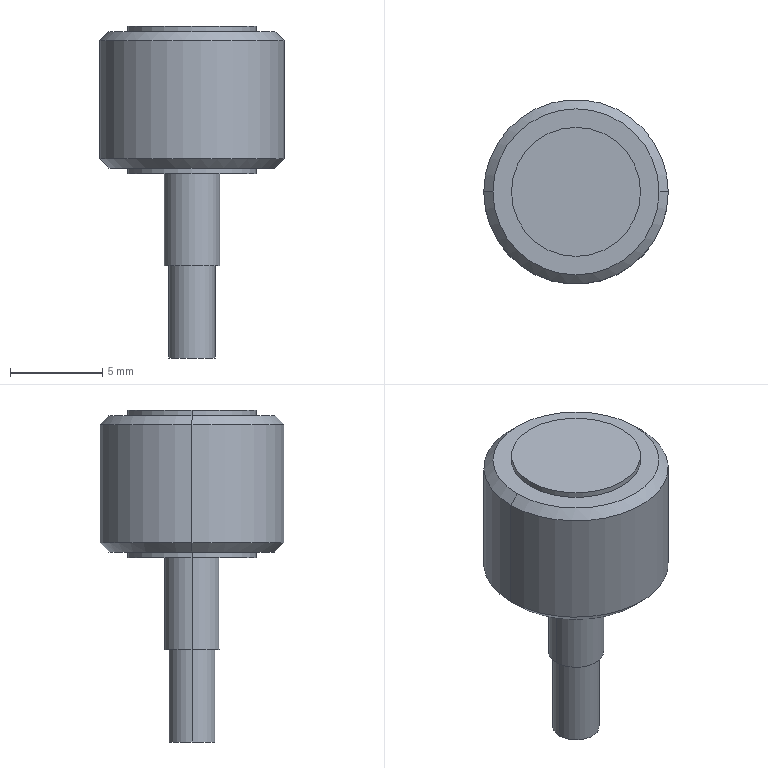Part | NX | 1 solid | 20 faces | box 10 x 10 x 18 mm | volume 656.58 mm3 | cylinder 10 | plane 6 | cone 4 | commonest cylinder face diameters 7 x4 2.5 x2 3 x2 10 x2
STEP:
#1=CARTESIAN_POINT('',(-3.5,0.,0.));
#2=VERTEX_POINT('',#1);
#3=CARTESIAN_POINT('',(3.5,0.,0.));
#4=VERTEX_POINT('',#3);
#5=CARTESIAN_POINT('',(0.,0.,0.));
#6=DIRECTION('',(0.,0.,1.));
#7=DIRECTION('',(1.,0.,0.));
#8=AXIS2_PLACEMENT_3D('',#5,#6,#7);
#9=CIRCLE('',#8,3.5);
#10=EDGE_CURVE('',#2,#4,#9,.T.);
#11=ORIENTED_EDGE('',*,*,#10,.F.);
#12=CARTESIAN_POINT('',(0.,0.,0.));
#13=DIRECTION('',(0.,0.,1.));
#14=DIRECTION('',(1.,0.,0.));
#15=AXIS2_PLACEMENT_3D('',#12,#13,#14);
#16=CIRCLE('',#15,3.5);
#17=EDGE_CURVE('',#4,#2,#16,.T.);
#18=ORIENTED_EDGE('',*,*,#17,.F.);
#19=EDGE_LOOP('',(#11,#18));
#20=FACE_BOUND('',#19,.T.);
#21=CARTESIAN_POINT('',(-1.5,0.,0.));
#22=VERTEX_POINT('',#21);
#23=CARTESIAN_POINT('',(1.5,0.,0.));
#24=VERTEX_POINT('',#23);
#25=CARTESIAN_POINT('',(0.,0.,0.));
#26=DIRECTION('',(0.,0.,-1.));
#27=DIRECTION('',(1.,0.,0.));
#28=AXIS2_PLACEMENT_3D('',#25,#26,#27);
#29=CIRCLE('',#28,1.5);
#30=EDGE_CURVE('',#22,#24,#29,.T.);
#31=ORIENTED_EDGE('',*,*,#30,.F.);
#32=CARTESIAN_POINT('',(0.,0.,0.));
#33=DIRECTION('',(0.,0.,-1.));
#34=DIRECTION('',(1.,0.,0.));
#35=AXIS2_PLACEMENT_3D('',#32,#33,#34);
#36=CIRCLE('',#35,1.5);
#37=EDGE_CURVE('',#24,#22,#36,.T.);
#38=ORIENTED_EDGE('',*,*,#37,.F.);
#39=EDGE_LOOP('',(#31,#38));
#40=FACE_BOUND('',#39,.T.);
#41=CARTESIAN_POINT('',(0.,0.,0.));
#42=DIRECTION('',(0.,0.,1.));
#43=DIRECTION('',(1.,0.,0.));
#44=AXIS2_PLACEMENT_3D('',#41,#42,#43);
#45=PLANE('',#44);
#46=ADVANCED_FACE('',(#20,#40),#45,.F.);
#47=CARTESIAN_POINT('',(3.5,0.,0.3));
#48=VERTEX_POINT('',#47);
#49=CARTESIAN_POINT('',(-3.5,0.,0.3));
#50=VERTEX_POINT('',#49);
#51=CARTESIAN_POINT('',(0.,0.,0.3));
#52=DIRECTION('',(0.,0.,-1.));
#53=DIRECTION('',(1.,0.,0.));
#54=AXIS2_PLACEMENT_3D('',#51,#52,#53);
#55=CIRCLE('',#54,3.5);
#56=EDGE_CURVE('',#48,#50,#55,.T.);
#57=ORIENTED_EDGE('',*,*,#56,.T.);
#58=CARTESIAN_POINT('',(-3.5,0.,8.4));
#59=DIRECTION('',(0.,0.,-1.));
#60=VECTOR('',#59,1000.);
#61=LINE('',#58,#60);
#62=EDGE_CURVE('',#50,#2,#61,.T.);
#63=ORIENTED_EDGE('',*,*,#62,.T.);
#64=ORIENTED_EDGE('',*,*,#10,.T.);
#65=CARTESIAN_POINT('',(3.5,0.,8.4));
#66=DIRECTION('',(0.,0.,-1.));
#67=VECTOR('',#66,1000.);
#68=LINE('',#65,#67);
#69=EDGE_CURVE('',#48,#4,#68,.T.);
#70=ORIENTED_EDGE('',*,*,#69,.F.);
#71=EDGE_LOOP('',(#57,#63,#64,#70));
#72=FACE_BOUND('',#71,.T.);
#73=CARTESIAN_POINT('',(0.,0.,8.4));
#74=DIRECTION('',(0.,0.,-1.));
#75=DIRECTION('',(1.,0.,0.));
#76=AXIS2_PLACEMENT_3D('',#73,#74,#75);
#77=CYLINDRICAL_SURFACE('',#76,3.5);
#78=ADVANCED_FACE('',(#72),#77,.T.);
#79=CARTESIAN_POINT('',(1.5,0.,-5.));
#80=VERTEX_POINT('',#79);
#81=CARTESIAN_POINT('',(-1.5,0.,-5.));
#82=VERTEX_POINT('',#81);
#83=CARTESIAN_POINT('',(0.,0.,-5.));
#84=DIRECTION('',(0.,0.,1.));
#85=DIRECTION('',(-1.,0.,0.));
#86=AXIS2_PLACEMENT_3D('',#83,#84,#85);
#87=CIRCLE('',#86,1.5);
#88=EDGE_CURVE('',#80,#82,#87,.T.);
#89=ORIENTED_EDGE('',*,*,#88,.F.);
#90=CARTESIAN_POINT('',(0.,0.,-5.));
#91=DIRECTION('',(0.,0.,1.));
#92=DIRECTION('',(-1.,0.,0.));
#93=AXIS2_PLACEMENT_3D('',#90,#91,#92);
#94=CIRCLE('',#93,1.5);
#95=EDGE_CURVE('',#82,#80,#94,.T.);
#96=ORIENTED_EDGE('',*,*,#95,.F.);
#97=EDGE_LOOP('',(#89,#96));
#98=FACE_BOUND('',#97,.T.);
#99=CARTESIAN_POINT('',(1.25,0.,-5.));
#100=VERTEX_POINT('',#99);
#101=CARTESIAN_POINT('',(-1.25,0.,-5.));
#102=VERTEX_POINT('',#101);
#103=CARTESIAN_POINT('',(0.,0.,-5.));
#104=DIRECTION('',(0.,0.,-1.));
#105=DIRECTION('',(1.,0.,0.));
#106=AXIS2_PLACEMENT_3D('',#103,#104,#105);
#107=CIRCLE('',#106,1.25);
#108=EDGE_CURVE('',#100,#102,#107,.T.);
#109=ORIENTED_EDGE('',*,*,#108,.F.);
#110=CARTESIAN_POINT('',(0.,0.,-5.));
#111=DIRECTION('',(0.,0.,-1.));
#112=DIRECTION('',(1.,0.,0.));
#113=AXIS2_PLACEMENT_3D('',#110,#111,#112);
#114=CIRCLE('',#113,1.25);
#115=EDGE_CURVE('',#102,#100,#114,.T.);
#116=ORIENTED_EDGE('',*,*,#115,.F.);
#117=EDGE_LOOP('',(#109,#116));
#118=FACE_BOUND('',#117,.T.);
#119=CARTESIAN_POINT('',(0.,0.,-5.));
#120=DIRECTION('',(0.,0.,-1.));
#121=DIRECTION('',(0.,-1.,0.));
#122=AXIS2_PLACEMENT_3D('',#119,#120,#121);
#123=PLANE('',#122);
#124=ADVANCED_FACE('',(#98,#118),#123,.T.);
#125=CARTESIAN_POINT('',(-4.5,0.,0.3));
#126=VERTEX_POINT('',#125);
#127=CARTESIAN_POINT('',(4.5,0.,0.3));
#128=VERTEX_POINT('',#127);
#129=CARTESIAN_POINT('',(0.,0.,0.3));
#130=DIRECTION('',(0.,0.,1.));
#131=DIRECTION('',(-1.,0.,0.));
#132=AXIS2_PLACEMENT_3D('',#129,#130,#131);
#133=CIRCLE('',#132,4.5);
#134=EDGE_CURVE('',#126,#128,#133,.T.);
#135=ORIENTED_EDGE('',*,*,#134,.F.);
#136=CARTESIAN_POINT('',(0.,0.,0.3));
#137=DIRECTION('',(0.,0.,1.));
#138=DIRECTION('',(-1.,0.,0.));
#139=AXIS2_PLACEMENT_3D('',#136,#137,#138);
#140=CIRCLE('',#139,4.5);
#141=EDGE_CURVE('',#128,#126,#140,.T.);
#142=ORIENTED_EDGE('',*,*,#141,.F.);
#143=EDGE_LOOP('',(#135,#142));
#144=FACE_BOUND('',#143,.T.);
#145=ORIENTED_EDGE('',*,*,#56,.F.);
#146=CARTESIAN_POINT('',(0.,0.,0.3));
#147=DIRECTION('',(0.,0.,-1.));
#148=DIRECTION('',(1.,0.,0.));
#149=AXIS2_PLACEMENT_3D('',#146,#147,#148);
#150=CIRCLE('',#149,3.5);
#151=EDGE_CURVE('',#50,#48,#150,.T.);
#152=ORIENTED_EDGE('',*,*,#151,.F.);
#153=EDGE_LOOP('',(#145,#152));
#154=FACE_BOUND('',#153,.T.);
#155=CARTESIAN_POINT('',(0.,0.,0.3));
#156=DIRECTION('',(0.,0.,-1.));
#157=DIRECTION('',(0.,-1.,0.));
#158=AXIS2_PLACEMENT_3D('',#155,#156,#157);
#159=PLANE('',#158);
#160=ADVANCED_FACE('',(#144,#154),#159,.T.);
#161=ORIENTED_EDGE('',*,*,#134,.T.);
#162=CARTESIAN_POINT('',(5.,0.,0.8));
#163=VERTEX_POINT('',#162);
#164=CARTESIAN_POINT('',(4.75,0.,0.55));
#165=DIRECTION('',(0.7071,0.,0.7071));
#166=VECTOR('',#165,1000.);
#167=LINE('',#164,#166);
#168=EDGE_CURVE('',#128,#163,#167,.T.);
#169=ORIENTED_EDGE('',*,*,#168,.T.);
#170=CARTESIAN_POINT('',(-5.,0.,0.8));
#171=VERTEX_POINT('',#170);
#172=CARTESIAN_POINT('',(0.,0.,0.8));
#173=DIRECTION('',(0.,0.,1.));
#174=DIRECTION('',(1.,0.,0.));
#175=AXIS2_PLACEMENT_3D('',#172,#173,#174);
#176=CIRCLE('',#175,5.);
#177=EDGE_CURVE('',#171,#163,#176,.T.);
#178=ORIENTED_EDGE('',*,*,#177,.F.);
#179=CARTESIAN_POINT('',(-4.75,0.,0.55));
#180=DIRECTION('',(-0.7071,0.,0.7071));
#181=VECTOR('',#180,1000.);
#182=LINE('',#179,#181);
#183=EDGE_CURVE('',#126,#171,#182,.T.);
#184=ORIENTED_EDGE('',*,*,#183,.F.);
#185=EDGE_LOOP('',(#161,#169,#178,#184));
#186=FACE_BOUND('',#185,.T.);
#187=CARTESIAN_POINT('',(0.,0.,0.55));
#188=DIRECTION('',(0.,0.,1.));
#189=DIRECTION('',(1.,0.,0.));
#190=AXIS2_PLACEMENT_3D('',#187,#188,#189);
#191=CONICAL_SURFACE('',#190,4.75,0.7854);
#192=ADVANCED_FACE('',(#186),#191,.T.);
#193=ORIENTED_EDGE('',*,*,#108,.T.);
#194=CARTESIAN_POINT('',(-1.25,0.,-10.));
#195=VERTEX_POINT('',#194);
#196=CARTESIAN_POINT('',(-1.25,0.,-5.));
#197=DIRECTION('',(0.,0.,-1.));
#198=VECTOR('',#197,1000.);
#199=LINE('',#196,#198);
#200=EDGE_CURVE('',#195,#102,#199,.F.);
#201=ORIENTED_EDGE('',*,*,#200,.F.);
#202=CARTESIAN_POINT('',(1.25,0.,-10.));
#203=VERTEX_POINT('',#202);
#204=CARTESIAN_POINT('',(0.,0.,-10.));
#205=DIRECTION('',(0.,0.,1.));
#206=DIRECTION('',(1.,0.,0.));
#207=AXIS2_PLACEMENT_3D('',#204,#205,#206);
#208=CIRCLE('',#207,1.25);
#209=EDGE_CURVE('',#195,#203,#208,.T.);
#210=ORIENTED_EDGE('',*,*,#209,.T.);
#211=CARTESIAN_POINT('',(1.25,0.,-5.));
#212=DIRECTION('',(0.,0.,-1.));
#213=VECTOR('',#212,1000.);
#214=LINE('',#211,#213);
#215=EDGE_CURVE('',#203,#100,#214,.F.);
#216=ORIENTED_EDGE('',*,*,#215,.T.);
#217=EDGE_LOOP('',(#193,#201,#210,#216));
#218=FACE_BOUND('',#217,.T.);
#219=CARTESIAN_POINT('',(0.,0.,-5.));
#220=DIRECTION('',(0.,0.,-1.));
#221=DIRECTION('',(-1.,0.,0.));
#222=AXIS2_PLACEMENT_3D('',#219,#220,#221);
#223=CYLINDRICAL_SURFACE('',#222,1.25);
#224=ADVANCED_FACE('',(#218),#223,.T.);
#225=CARTESIAN_POINT('',(-5.,0.,7.2));
#226=VERTEX_POINT('',#225);
#227=CARTESIAN_POINT('',(5.,0.,7.2));
#228=VERTEX_POINT('',#227);
#229=CARTESIAN_POINT('',(0.,0.,7.2));
#230=DIRECTION('',(0.,0.,-1.));
#231=DIRECTION('',(1.,0.,0.));
#232=AXIS2_PLACEMENT_3D('',#229,#230,#231);
#233=CIRCLE('',#232,5.);
#234=EDGE_CURVE('',#226,#228,#233,.T.);
#235=ORIENTED_EDGE('',*,*,#234,.T.);
#236=CARTESIAN_POINT('',(5.,0.,0.));
#237=DIRECTION('',(0.,0.,1.));
#238=VECTOR('',#237,1000.);
#239=LINE('',#236,#238);
#240=EDGE_CURVE('',#163,#228,#239,.T.);
#241=ORIENTED_EDGE('',*,*,#240,.F.);
#242=CARTESIAN_POINT('',(0.,0.,0.8));
#243=DIRECTION('',(0.,0.,1.));
#244=DIRECTION('',(1.,0.,0.));
#245=AXIS2_PLACEMENT_3D('',#242,#243,#244);
#246=CIRCLE('',#245,5.);
#247=EDGE_CURVE('',#163,#171,#246,.T.);
#248=ORIENTED_EDGE('',*,*,#247,.T.);
#249=CARTESIAN_POINT('',(-5.,0.,0.));
#250=DIRECTION('',(0.,0.,1.));
#251=VECTOR('',#250,1000.);
#252=LINE('',#249,#251);
#253=EDGE_CURVE('',#171,#226,#252,.T.);
#254=ORIENTED_EDGE('',*,*,#253,.T.);
#255=EDGE_LOOP('',(#235,#241,#248,#254));
#256=FACE_BOUND('',#255,.T.);
#257=CARTESIAN_POINT('',(0.,0.,0.));
#258=DIRECTION('',(0.,0.,1.));
#259=DIRECTION('',(1.,0.,0.));
#260=AXIS2_PLACEMENT_3D('',#257,#258,#259);
#261=CYLINDRICAL_SURFACE('',#260,5.);
#262=ADVANCED_FACE('',(#256),#261,.T.);
#263=ORIENTED_EDGE('',*,*,#209,.F.);
#264=CARTESIAN_POINT('',(0.,0.,-10.));
#265=DIRECTION('',(0.,0.,1.));
#266=DIRECTION('',(1.,0.,0.));
#267=AXIS2_PLACEMENT_3D('',#264,#265,#266);
#268=CIRCLE('',#267,1.25);
#269=EDGE_CURVE('',#203,#195,#268,.T.);
#270=ORIENTED_EDGE('',*,*,#269,.F.);
#271=EDGE_LOOP('',(#263,#270));
#272=FACE_BOUND('',#271,.T.);
#273=CARTESIAN_POINT('',(0.,0.,-10.));
#274=DIRECTION('',(0.,0.,-1.));
#275=DIRECTION('',(0.,-1.,0.));
#276=AXIS2_PLACEMENT_3D('',#273,#274,#275);
#277=PLANE('',#276);
#278=ADVANCED_FACE('',(#272),#277,.T.);
#279=CARTESIAN_POINT('',(-4.5,0.,7.7));
#280=VERTEX_POINT('',#279);
#281=CARTESIAN_POINT('',(4.5,0.,7.7));
#282=VERTEX_POINT('',#281);
#283=CARTESIAN_POINT('',(0.,0.,7.7));
#284=DIRECTION('',(0.,0.,-1.));
#285=DIRECTION('',(1.,0.,0.));
#286=AXIS2_PLACEMENT_3D('',#283,#284,#285);
#287=CIRCLE('',#286,4.5);
#288=EDGE_CURVE('',#280,#282,#287,.T.);
#289=ORIENTED_EDGE('',*,*,#288,.T.);
#290=CARTESIAN_POINT('',(4.75,0.,7.45));
#291=DIRECTION('',(0.7071,0.,-0.7071));
#292=VECTOR('',#291,1000.);
#293=LINE('',#290,#292);
#294=EDGE_CURVE('',#228,#282,#293,.F.);
#295=ORIENTED_EDGE('',*,*,#294,.F.);
#296=ORIENTED_EDGE('',*,*,#234,.F.);
#297=CARTESIAN_POINT('',(-4.75,0.,7.45));
#298=DIRECTION('',(-0.7071,0.,-0.7071));
#299=VECTOR('',#298,1000.);
#300=LINE('',#297,#299);
#301=EDGE_CURVE('',#226,#280,#300,.F.);
#302=ORIENTED_EDGE('',*,*,#301,.T.);
#303=EDGE_LOOP('',(#289,#295,#296,#302));
#304=FACE_BOUND('',#303,.T.);
#305=CARTESIAN_POINT('',(0.,0.,7.45));
#306=DIRECTION('',(0.,0.,-1.));
#307=DIRECTION('',(-1.,0.,0.));
#308=AXIS2_PLACEMENT_3D('',#305,#306,#307);
#309=CONICAL_SURFACE('',#308,4.75,0.7854);
#310=ADVANCED_FACE('',(#304),#309,.T.);
#311=ORIENTED_EDGE('',*,*,#288,.F.);
#312=CARTESIAN_POINT('',(0.,0.,7.7));
#313=DIRECTION('',(0.,0.,-1.));
#314=DIRECTION('',(1.,0.,0.));
#315=AXIS2_PLACEMENT_3D('',#312,#313,#314);
#316=CIRCLE('',#315,4.5);
#317=EDGE_CURVE('',#282,#280,#316,.T.);
#318=ORIENTED_EDGE('',*,*,#317,.F.);
#319=EDGE_LOOP('',(#311,#318));
#320=FACE_BOUND('',#319,.T.);
#321=CARTESIAN_POINT('',(3.5,0.,7.7));
#322=VERTEX_POINT('',#321);
#323=CARTESIAN_POINT('',(-3.5,0.,7.7));
#324=VERTEX_POINT('',#323);
#325=CARTESIAN_POINT('',(0.,0.,7.7));
#326=DIRECTION('',(0.,0.,1.));
#327=DIRECTION('',(-1.,0.,0.));
#328=AXIS2_PLACEMENT_3D('',#325,#326,#327);
#329=CIRCLE('',#328,3.5);
#330=EDGE_CURVE('',#322,#324,#329,.T.);
#331=ORIENTED_EDGE('',*,*,#330,.F.);
#332=CARTESIAN_POINT('',(0.,0.,7.7));
#333=DIRECTION('',(0.,0.,1.));
#334=DIRECTION('',(-1.,0.,0.));
#335=AXIS2_PLACEMENT_3D('',#332,#333,#334);
#336=CIRCLE('',#335,3.5);
#337=EDGE_CURVE('',#324,#322,#336,.T.);
#338=ORIENTED_EDGE('',*,*,#337,.F.);
#339=EDGE_LOOP('',(#331,#338));
#340=FACE_BOUND('',#339,.T.);
#341=CARTESIAN_POINT('',(0.,0.,7.7));
#342=DIRECTION('',(0.,0.,-1.));
#343=DIRECTION('',(0.,-1.,0.));
#344=AXIS2_PLACEMENT_3D('',#341,#342,#343);
#345=PLANE('',#344);
#346=ADVANCED_FACE('',(#320,#340),#345,.F.);
#347=ORIENTED_EDGE('',*,*,#30,.T.);
#348=CARTESIAN_POINT('',(1.5,0.,0.));
#349=DIRECTION('',(0.,0.,-1.));
#350=VECTOR('',#349,1000.);
#351=LINE('',#348,#350);
#352=EDGE_CURVE('',#80,#24,#351,.F.);
#353=ORIENTED_EDGE('',*,*,#352,.F.);
#354=ORIENTED_EDGE('',*,*,#88,.T.);
#355=CARTESIAN_POINT('',(-1.5,0.,0.));
#356=DIRECTION('',(0.,0.,-1.));
#357=VECTOR('',#356,1000.);
#358=LINE('',#355,#357);
#359=EDGE_CURVE('',#82,#22,#358,.F.);
#360=ORIENTED_EDGE('',*,*,#359,.T.);
#361=EDGE_LOOP('',(#347,#353,#354,#360));
#362=FACE_BOUND('',#361,.T.);
#363=CARTESIAN_POINT('',(0.,0.,0.));
#364=DIRECTION('',(0.,0.,-1.));
#365=DIRECTION('',(-1.,0.,0.));
#366=AXIS2_PLACEMENT_3D('',#363,#364,#365);
#367=CYLINDRICAL_SURFACE('',#366,1.5);
#368=ADVANCED_FACE('',(#362),#367,.T.);
#369=CARTESIAN_POINT('',(-3.5,0.,8.));
#370=VERTEX_POINT('',#369);
#371=CARTESIAN_POINT('',(3.5,0.,8.));
#372=VERTEX_POINT('',#371);
#373=CARTESIAN_POINT('',(0.,0.,8.));
#374=DIRECTION('',(0.,0.,-1.));
#375=DIRECTION('',(1.,0.,0.));
#376=AXIS2_PLACEMENT_3D('',#373,#374,#375);
#377=CIRCLE('',#376,3.5);
#378=EDGE_CURVE('',#370,#372,#377,.T.);
#379=ORIENTED_EDGE('',*,*,#378,.T.);
#380=CARTESIAN_POINT('',(3.5,0.,8.4));
#381=DIRECTION('',(0.,0.,-1.));
#382=VECTOR('',#381,1000.);
#383=LINE('',#380,#382);
#384=EDGE_CURVE('',#372,#322,#383,.T.);
#385=ORIENTED_EDGE('',*,*,#384,.T.);
#386=ORIENTED_EDGE('',*,*,#330,.T.);
#387=CARTESIAN_POINT('',(-3.5,0.,8.4));
#388=DIRECTION('',(0.,0.,-1.));
#389=VECTOR('',#388,1000.);
#390=LINE('',#387,#389);
#391=EDGE_CURVE('',#370,#324,#390,.T.);
#392=ORIENTED_EDGE('',*,*,#391,.F.);
#393=EDGE_LOOP('',(#379,#385,#386,#392));
#394=FACE_BOUND('',#393,.T.);
#395=CARTESIAN_POINT('',(0.,0.,8.4));
#396=DIRECTION('',(0.,0.,-1.));
#397=DIRECTION('',(1.,0.,0.));
#398=AXIS2_PLACEMENT_3D('',#395,#396,#397);
#399=CYLINDRICAL_SURFACE('',#398,3.5);
#400=ADVANCED_FACE('',(#394),#399,.T.);
#401=ORIENTED_EDGE('',*,*,#378,.F.);
#402=CARTESIAN_POINT('',(0.,0.,8.));
#403=DIRECTION('',(0.,0.,-1.));
#404=DIRECTION('',(1.,0.,0.));
#405=AXIS2_PLACEMENT_3D('',#402,#403,#404);
#406=CIRCLE('',#405,3.5);
#407=EDGE_CURVE('',#372,#370,#406,.T.);
#408=ORIENTED_EDGE('',*,*,#407,.F.);
#409=EDGE_LOOP('',(#401,#408));
#410=FACE_BOUND('',#409,.T.);
#411=CARTESIAN_POINT('',(0.,0.,8.));
#412=DIRECTION('',(0.,0.,1.));
#413=DIRECTION('',(1.,0.,0.));
#414=AXIS2_PLACEMENT_3D('',#411,#412,#413);
#415=PLANE('',#414);
#416=ADVANCED_FACE('',(#410),#415,.T.);
#417=ORIENTED_EDGE('',*,*,#359,.F.);
#418=ORIENTED_EDGE('',*,*,#95,.T.);
#419=ORIENTED_EDGE('',*,*,#352,.T.);
#420=ORIENTED_EDGE('',*,*,#37,.T.);
#421=EDGE_LOOP('',(#417,#418,#419,#420));
#422=FACE_BOUND('',#421,.T.);
#423=CARTESIAN_POINT('',(0.,0.,0.));
#424=DIRECTION('',(0.,0.,-1.));
#425=DIRECTION('',(-1.,0.,0.));
#426=AXIS2_PLACEMENT_3D('',#423,#424,#425);
#427=CYLINDRICAL_SURFACE('',#426,1.5);
#428=ADVANCED_FACE('',(#422),#427,.T.);
#429=ORIENTED_EDGE('',*,*,#247,.F.);
#430=ORIENTED_EDGE('',*,*,#168,.F.);
#431=ORIENTED_EDGE('',*,*,#141,.T.);
#432=ORIENTED_EDGE('',*,*,#183,.T.);
#433=EDGE_LOOP('',(#429,#430,#431,#432));
#434=FACE_BOUND('',#433,.T.);
#435=CARTESIAN_POINT('',(0.,0.,0.55));
#436=DIRECTION('',(0.,0.,1.));
#437=DIRECTION('',(1.,0.,0.));
#438=AXIS2_PLACEMENT_3D('',#435,#436,#437);
#439=CONICAL_SURFACE('',#438,4.75,0.7854);
#440=ADVANCED_FACE('',(#434),#439,.T.);
#441=ORIENTED_EDGE('',*,*,#384,.F.);
#442=ORIENTED_EDGE('',*,*,#407,.T.);
#443=ORIENTED_EDGE('',*,*,#391,.T.);
#444=ORIENTED_EDGE('',*,*,#337,.T.);
#445=EDGE_LOOP('',(#441,#442,#443,#444));
#446=FACE_BOUND('',#445,.T.);
#447=CARTESIAN_POINT('',(0.,0.,8.4));
#448=DIRECTION('',(0.,0.,-1.));
#449=DIRECTION('',(1.,0.,0.));
#450=AXIS2_PLACEMENT_3D('',#447,#448,#449);
#451=CYLINDRICAL_SURFACE('',#450,3.5);
#452=ADVANCED_FACE('',(#446),#451,.T.);
#453=ORIENTED_EDGE('',*,*,#240,.T.);
#454=CARTESIAN_POINT('',(0.,0.,7.2));
#455=DIRECTION('',(0.,0.,-1.));
#456=DIRECTION('',(1.,0.,0.));
#457=AXIS2_PLACEMENT_3D('',#454,#455,#456);
#458=CIRCLE('',#457,5.);
#459=EDGE_CURVE('',#228,#226,#458,.T.);
#460=ORIENTED_EDGE('',*,*,#459,.T.);
#461=ORIENTED_EDGE('',*,*,#253,.F.);
#462=ORIENTED_EDGE('',*,*,#177,.T.);
#463=EDGE_LOOP('',(#453,#460,#461,#462));
#464=FACE_BOUND('',#463,.T.);
#465=CARTESIAN_POINT('',(0.,0.,0.));
#466=DIRECTION('',(0.,0.,1.));
#467=DIRECTION('',(1.,0.,0.));
#468=AXIS2_PLACEMENT_3D('',#465,#466,#467);
#469=CYLINDRICAL_SURFACE('',#468,5.);
#470=ADVANCED_FACE('',(#464),#469,.T.);
#471=ORIENTED_EDGE('',*,*,#69,.T.);
#472=ORIENTED_EDGE('',*,*,#17,.T.);
#473=ORIENTED_EDGE('',*,*,#62,.F.);
#474=ORIENTED_EDGE('',*,*,#151,.T.);
#475=EDGE_LOOP('',(#471,#472,#473,#474));
#476=FACE_BOUND('',#475,.T.);
#477=CARTESIAN_POINT('',(0.,0.,8.4));
#478=DIRECTION('',(0.,0.,-1.));
#479=DIRECTION('',(1.,0.,0.));
#480=AXIS2_PLACEMENT_3D('',#477,#478,#479);
#481=CYLINDRICAL_SURFACE('',#480,3.5);
#482=ADVANCED_FACE('',(#476),#481,.T.);
#483=ORIENTED_EDGE('',*,*,#200,.T.);
#484=ORIENTED_EDGE('',*,*,#115,.T.);
#485=ORIENTED_EDGE('',*,*,#215,.F.);
#486=ORIENTED_EDGE('',*,*,#269,.T.);
#487=EDGE_LOOP('',(#483,#484,#485,#486));
#488=FACE_BOUND('',#487,.T.);
#489=CARTESIAN_POINT('',(0.,0.,-5.));
#490=DIRECTION('',(0.,0.,-1.));
#491=DIRECTION('',(-1.,0.,0.));
#492=AXIS2_PLACEMENT_3D('',#489,#490,#491);
#493=CYLINDRICAL_SURFACE('',#492,1.25);
#494=ADVANCED_FACE('',(#488),#493,.T.);
#495=ORIENTED_EDGE('',*,*,#301,.F.);
#496=ORIENTED_EDGE('',*,*,#459,.F.);
#497=ORIENTED_EDGE('',*,*,#294,.T.);
#498=ORIENTED_EDGE('',*,*,#317,.T.);
#499=EDGE_LOOP('',(#495,#496,#497,#498));
#500=FACE_BOUND('',#499,.T.);
#501=CARTESIAN_POINT('',(0.,0.,7.45));
#502=DIRECTION('',(0.,0.,-1.));
#503=DIRECTION('',(-1.,0.,0.));
#504=AXIS2_PLACEMENT_3D('',#501,#502,#503);
#505=CONICAL_SURFACE('',#504,4.75,0.7854);
#506=ADVANCED_FACE('',(#500),#505,.T.);
#507=CLOSED_SHELL('',(#46,#78,#124,#160,#192,#224,#262,#278,#310,#346,#368,#400,#416,#428,#440,#452,#470,#482,#494,#506));
#508=MANIFOLD_SOLID_BREP('',#507);
#509=(LENGTH_UNIT()NAMED_UNIT(*)SI_UNIT(.MILLI.,.METRE.));
#510=UNCERTAINTY_MEASURE_WITH_UNIT(LENGTH_MEASURE(0.00001),#509,'','');
#511=(NAMED_UNIT(*)PLANE_ANGLE_UNIT()SI_UNIT($,.RADIAN.));
#512=(NAMED_UNIT(*)SI_UNIT($,.STERADIAN.)SOLID_ANGLE_UNIT());
#513=(GEOMETRIC_REPRESENTATION_CONTEXT(3)GLOBAL_UNCERTAINTY_ASSIGNED_CONTEXT((#510))GLOBAL_UNIT_ASSIGNED_CONTEXT((#509,#511,#512))REPRESENTATION_CONTEXT('',''));
#514=ADVANCED_BREP_SHAPE_REPRESENTATION('',(#508),#513);